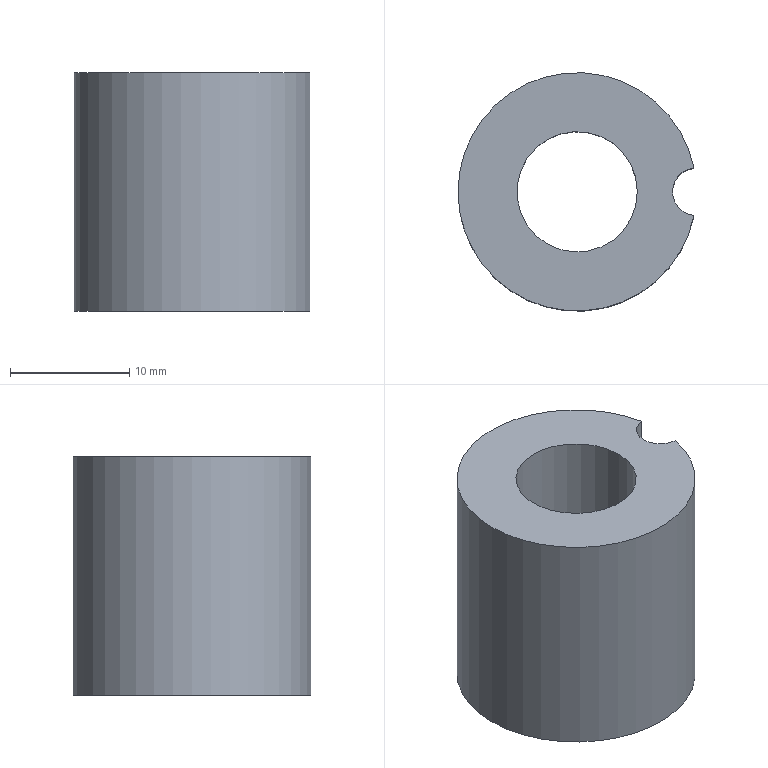Part | NX | features solid 2 | 1 solid | 7 faces | box 19.8 x 20 x 20 mm | volume 4026 mm3 | cylinder 4 | plane 3 | commonest cylinder face diameters 4 x1 10.1 x1 12.6 x1 20 x1
STEP:
#1=CARTESIAN_POINT('',(294.8,245.183,6.603));
#2=VERTEX_POINT('',#1);
#3=CARTESIAN_POINT('',(294.8,245.183,26.603));
#4=VERTEX_POINT('',#3);
#5=CARTESIAN_POINT('',(294.8,245.183,16.603));
#6=DIRECTION('',(0.,0.,1.));
#7=VECTOR('',#6,1000.);
#8=LINE('',#5,#7);
#9=EDGE_CURVE('',#2,#4,#8,.T.);
#10=ORIENTED_EDGE('',*,*,#9,.F.);
#11=CARTESIAN_POINT('',(294.8,241.203,6.603));
#12=VERTEX_POINT('',#11);
#13=CARTESIAN_POINT('',(285.,243.193,6.603));
#14=DIRECTION('',(0.,0.,1.));
#15=DIRECTION('',(1.,0.,0.));
#16=AXIS2_PLACEMENT_3D('',#13,#14,#15);
#17=CIRCLE('',#16,10.);
#18=EDGE_CURVE('',#2,#12,#17,.T.);
#19=ORIENTED_EDGE('',*,*,#18,.T.);
#20=CARTESIAN_POINT('',(294.8,241.203,26.603));
#21=VERTEX_POINT('',#20);
#22=CARTESIAN_POINT('',(294.8,241.203,16.603));
#23=DIRECTION('',(0.,0.,1.));
#24=VECTOR('',#23,1000.);
#25=LINE('',#22,#24);
#26=EDGE_CURVE('',#21,#12,#25,.F.);
#27=ORIENTED_EDGE('',*,*,#26,.F.);
#28=CARTESIAN_POINT('',(285.,243.193,26.603));
#29=DIRECTION('',(0.,0.,1.));
#30=DIRECTION('',(1.,0.,0.));
#31=AXIS2_PLACEMENT_3D('',#28,#29,#30);
#32=CIRCLE('',#31,10.);
#33=EDGE_CURVE('',#4,#21,#32,.T.);
#34=ORIENTED_EDGE('',*,*,#33,.F.);
#35=EDGE_LOOP('',(#10,#19,#27,#34));
#36=FACE_BOUND('',#35,.T.);
#37=CARTESIAN_POINT('',(285.,243.193,6.603));
#38=DIRECTION('',(0.,0.,1.));
#39=DIRECTION('',(1.,0.,0.));
#40=AXIS2_PLACEMENT_3D('',#37,#38,#39);
#41=CYLINDRICAL_SURFACE('',#40,10.);
#42=ADVANCED_FACE('',(#36),#41,.T.);
#43=CARTESIAN_POINT('',(291.3,243.193,6.603));
#44=VERTEX_POINT('',#43);
#45=CARTESIAN_POINT('',(285.,243.193,6.603));
#46=DIRECTION('',(0.,0.,1.));
#47=DIRECTION('',(1.,0.,0.));
#48=AXIS2_PLACEMENT_3D('',#45,#46,#47);
#49=CIRCLE('',#48,6.3);
#50=EDGE_CURVE('',#44,#44,#49,.T.);
#51=ORIENTED_EDGE('',*,*,#50,.T.);
#52=EDGE_LOOP('',(#51));
#53=FACE_BOUND('',#52,.T.);
#54=ORIENTED_EDGE('',*,*,#18,.F.);
#55=CARTESIAN_POINT('',(295.,243.193,6.603));
#56=DIRECTION('',(0.,0.,1.));
#57=DIRECTION('',(1.,0.,0.));
#58=AXIS2_PLACEMENT_3D('',#55,#56,#57);
#59=CIRCLE('',#58,2.);
#60=EDGE_CURVE('',#2,#12,#59,.T.);
#61=ORIENTED_EDGE('',*,*,#60,.T.);
#62=EDGE_LOOP('',(#54,#61));
#63=FACE_BOUND('',#62,.T.);
#64=CARTESIAN_POINT('',(285.,243.193,6.603));
#65=DIRECTION('',(0.,0.,1.));
#66=DIRECTION('',(1.,0.,0.));
#67=AXIS2_PLACEMENT_3D('',#64,#65,#66);
#68=PLANE('',#67);
#69=ADVANCED_FACE('',(#53,#63),#68,.F.);
#70=CARTESIAN_POINT('',(290.05,243.193,26.603));
#71=VERTEX_POINT('',#70);
#72=CARTESIAN_POINT('',(285.,243.193,26.603));
#73=DIRECTION('',(0.,0.,1.));
#74=DIRECTION('',(1.,0.,0.));
#75=AXIS2_PLACEMENT_3D('',#72,#73,#74);
#76=CIRCLE('',#75,5.05);
#77=EDGE_CURVE('',#71,#71,#76,.T.);
#78=ORIENTED_EDGE('',*,*,#77,.F.);
#79=EDGE_LOOP('',(#78));
#80=FACE_BOUND('',#79,.T.);
#81=CARTESIAN_POINT('',(295.,243.193,26.603));
#82=DIRECTION('',(0.,0.,1.));
#83=DIRECTION('',(1.,0.,0.));
#84=AXIS2_PLACEMENT_3D('',#81,#82,#83);
#85=CIRCLE('',#84,2.);
#86=EDGE_CURVE('',#4,#21,#85,.T.);
#87=ORIENTED_EDGE('',*,*,#86,.F.);
#88=ORIENTED_EDGE('',*,*,#33,.T.);
#89=EDGE_LOOP('',(#87,#88));
#90=FACE_BOUND('',#89,.T.);
#91=CARTESIAN_POINT('',(285.,243.193,26.603));
#92=DIRECTION('',(0.,0.,1.));
#93=DIRECTION('',(1.,0.,0.));
#94=AXIS2_PLACEMENT_3D('',#91,#92,#93);
#95=PLANE('',#94);
#96=ADVANCED_FACE('',(#80,#90),#95,.T.);
#97=ORIENTED_EDGE('',*,*,#50,.F.);
#98=EDGE_LOOP('',(#97));
#99=FACE_BOUND('',#98,.T.);
#100=CARTESIAN_POINT('',(291.3,243.193,18.603));
#101=VERTEX_POINT('',#100);
#102=CARTESIAN_POINT('',(285.,243.193,18.603));
#103=DIRECTION('',(0.,0.,1.));
#104=DIRECTION('',(1.,0.,0.));
#105=AXIS2_PLACEMENT_3D('',#102,#103,#104);
#106=CIRCLE('',#105,6.3);
#107=EDGE_CURVE('',#101,#101,#106,.T.);
#108=ORIENTED_EDGE('',*,*,#107,.T.);
#109=EDGE_LOOP('',(#108));
#110=FACE_BOUND('',#109,.T.);
#111=CARTESIAN_POINT('',(285.,243.193,6.603));
#112=DIRECTION('',(0.,0.,1.));
#113=DIRECTION('',(1.,0.,0.));
#114=AXIS2_PLACEMENT_3D('',#111,#112,#113);
#115=CYLINDRICAL_SURFACE('',#114,6.3);
#116=ADVANCED_FACE('',(#99,#110),#115,.F.);
#117=CARTESIAN_POINT('',(290.05,243.193,18.603));
#118=VERTEX_POINT('',#117);
#119=CARTESIAN_POINT('',(285.,243.193,18.603));
#120=DIRECTION('',(0.,0.,1.));
#121=DIRECTION('',(1.,0.,0.));
#122=AXIS2_PLACEMENT_3D('',#119,#120,#121);
#123=CIRCLE('',#122,5.05);
#124=EDGE_CURVE('',#118,#118,#123,.T.);
#125=ORIENTED_EDGE('',*,*,#124,.T.);
#126=EDGE_LOOP('',(#125));
#127=FACE_BOUND('',#126,.T.);
#128=ORIENTED_EDGE('',*,*,#107,.F.);
#129=EDGE_LOOP('',(#128));
#130=FACE_BOUND('',#129,.T.);
#131=CARTESIAN_POINT('',(285.,243.193,18.603));
#132=DIRECTION('',(0.,0.,1.));
#133=DIRECTION('',(1.,0.,0.));
#134=AXIS2_PLACEMENT_3D('',#131,#132,#133);
#135=PLANE('',#134);
#136=ADVANCED_FACE('',(#127,#130),#135,.F.);
#137=ORIENTED_EDGE('',*,*,#9,.T.);
#138=ORIENTED_EDGE('',*,*,#86,.T.);
#139=ORIENTED_EDGE('',*,*,#26,.T.);
#140=ORIENTED_EDGE('',*,*,#60,.F.);
#141=EDGE_LOOP('',(#137,#138,#139,#140));
#142=FACE_BOUND('',#141,.T.);
#143=CARTESIAN_POINT('',(295.,243.193,6.603));
#144=DIRECTION('',(0.,0.,1.));
#145=DIRECTION('',(1.,0.,0.));
#146=AXIS2_PLACEMENT_3D('',#143,#144,#145);
#147=CYLINDRICAL_SURFACE('',#146,2.);
#148=ADVANCED_FACE('',(#142),#147,.F.);
#149=ORIENTED_EDGE('',*,*,#77,.T.);
#150=EDGE_LOOP('',(#149));
#151=FACE_BOUND('',#150,.T.);
#152=ORIENTED_EDGE('',*,*,#124,.F.);
#153=EDGE_LOOP('',(#152));
#154=FACE_BOUND('',#153,.T.);
#155=CARTESIAN_POINT('',(285.,243.193,6.603));
#156=DIRECTION('',(0.,0.,1.));
#157=DIRECTION('',(1.,0.,0.));
#158=AXIS2_PLACEMENT_3D('',#155,#156,#157);
#159=CYLINDRICAL_SURFACE('',#158,5.05);
#160=ADVANCED_FACE('',(#151,#154),#159,.F.);
#161=CLOSED_SHELL('',(#42,#69,#96,#116,#136,#148,#160));
#162=MANIFOLD_SOLID_BREP('',#161);
#163=(LENGTH_UNIT()NAMED_UNIT(*)SI_UNIT(.MILLI.,.METRE.));
#164=UNCERTAINTY_MEASURE_WITH_UNIT(LENGTH_MEASURE(0.00001),#163,'','');
#165=(NAMED_UNIT(*)PLANE_ANGLE_UNIT()SI_UNIT($,.RADIAN.));
#166=(NAMED_UNIT(*)SI_UNIT($,.STERADIAN.)SOLID_ANGLE_UNIT());
#167=(GEOMETRIC_REPRESENTATION_CONTEXT(3)GLOBAL_UNCERTAINTY_ASSIGNED_CONTEXT((#164))GLOBAL_UNIT_ASSIGNED_CONTEXT((#163,#165,#166))REPRESENTATION_CONTEXT('',''));
#168=ADVANCED_BREP_SHAPE_REPRESENTATION('',(#162),#167);